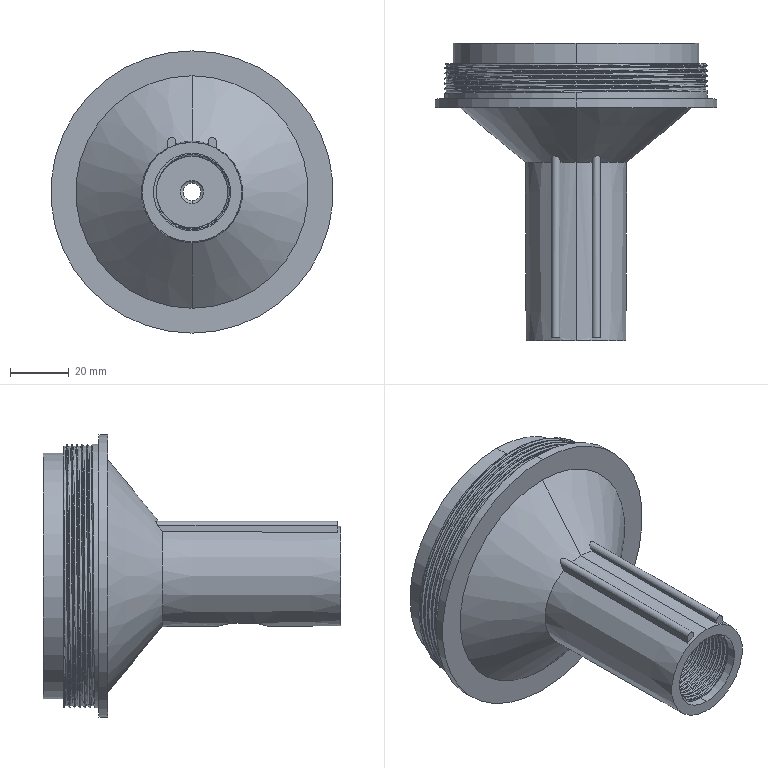Part | SolidWorks | features ICE 6, Helix 2, SweepCut 2, Revolution 1 | 1 solid | 133 faces | box 96.5 x 101.609 x 96.5 mm | volume 64001 mm3 | cylinder 85 | plane 28 | cone 12 | spline 6 | torus 2 | commonest cylinder face diameters 24.5 x26 90.1 x13 3.3 x12 8 x12 2.2 x8 2.8 x2